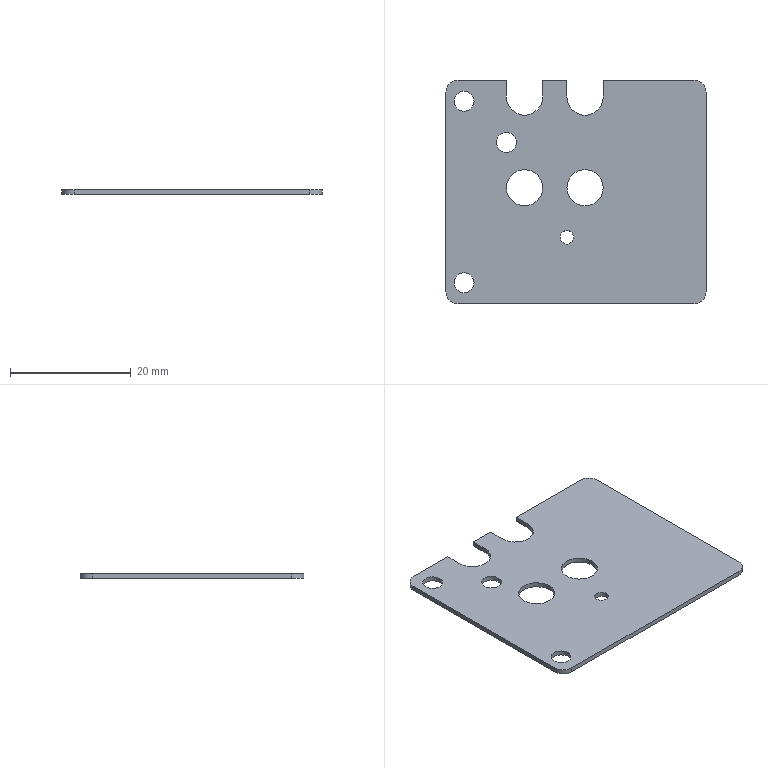Part | SolidWorks | features ICE 5, HoleWzd 2, Cut 1, Extrusion 1, Fillet 1, MirrorPattern 1, MoveFace 1 | 1 solid | 30 faces | box 43 x 37 x 0.8 mm | volume 1152 mm3 | cylinder 18 | plane 12 | commonest cylinder face diameters 3.3 x6 6 x6 4 x4 2.25 x2
STEP:
#1=CARTESIAN_POINT('',(-13.15,8.2,0.));
#2=VERTEX_POINT('',#1);
#3=CARTESIAN_POINT('',(-9.85,8.2,0.));
#4=VERTEX_POINT('',#3);
#5=CARTESIAN_POINT('',(-11.5,8.2,0.));
#6=DIRECTION('',(0.,0.,1.));
#7=DIRECTION('',(1.,0.,0.));
#8=AXIS2_PLACEMENT_3D('',#5,#6,#7);
#9=CIRCLE('',#8,1.65);
#10=EDGE_CURVE('',#2,#4,#9,.T.);
#11=ORIENTED_EDGE('',*,*,#10,.F.);
#12=CARTESIAN_POINT('',(-13.15,8.2,0.8));
#13=VERTEX_POINT('',#12);
#14=CARTESIAN_POINT('',(-13.15,8.2,-29.2));
#15=DIRECTION('',(0.,0.,1.));
#16=VECTOR('',#15,1000.);
#17=LINE('',#14,#16);
#18=EDGE_CURVE('',#2,#13,#17,.T.);
#19=ORIENTED_EDGE('',*,*,#18,.T.);
#20=CARTESIAN_POINT('',(-9.85,8.2,0.8));
#21=VERTEX_POINT('',#20);
#22=CARTESIAN_POINT('',(-11.5,8.2,0.8));
#23=DIRECTION('',(0.,0.,1.));
#24=DIRECTION('',(1.,0.,0.));
#25=AXIS2_PLACEMENT_3D('',#22,#23,#24);
#26=CIRCLE('',#25,1.65);
#27=EDGE_CURVE('',#13,#21,#26,.T.);
#28=ORIENTED_EDGE('',*,*,#27,.T.);
#29=CARTESIAN_POINT('',(-9.85,8.2,-29.2));
#30=DIRECTION('',(0.,0.,1.));
#31=VECTOR('',#30,1000.);
#32=LINE('',#29,#31);
#33=EDGE_CURVE('',#4,#21,#32,.T.);
#34=ORIENTED_EDGE('',*,*,#33,.F.);
#35=EDGE_LOOP('',(#11,#19,#28,#34));
#36=FACE_OUTER_BOUND('',#35,.T.);
#37=CARTESIAN_POINT('',(-11.5,8.2,-29.2));
#38=DIRECTION('',(0.,0.,1.));
#39=DIRECTION('',(1.,0.,0.));
#40=AXIS2_PLACEMENT_3D('',#37,#38,#39);
#41=CYLINDRICAL_SURFACE('',#40,1.65);
#42=ADVANCED_FACE('',(#36),#41,.F.);
#43=CARTESIAN_POINT('',(-20.15,15.,0.));
#44=VERTEX_POINT('',#43);
#45=CARTESIAN_POINT('',(-16.85,15.,0.));
#46=VERTEX_POINT('',#45);
#47=CARTESIAN_POINT('',(-18.5,15.,0.));
#48=DIRECTION('',(0.,0.,1.));
#49=DIRECTION('',(1.,0.,0.));
#50=AXIS2_PLACEMENT_3D('',#47,#48,#49);
#51=CIRCLE('',#50,1.65);
#52=EDGE_CURVE('',#44,#46,#51,.T.);
#53=ORIENTED_EDGE('',*,*,#52,.F.);
#54=CARTESIAN_POINT('',(-20.15,15.,0.8));
#55=VERTEX_POINT('',#54);
#56=CARTESIAN_POINT('',(-20.15,15.,0.8));
#57=DIRECTION('',(0.,0.,1.));
#58=VECTOR('',#57,1000.);
#59=LINE('',#56,#58);
#60=EDGE_CURVE('',#44,#55,#59,.T.);
#61=ORIENTED_EDGE('',*,*,#60,.T.);
#62=CARTESIAN_POINT('',(-16.85,15.,0.8));
#63=VERTEX_POINT('',#62);
#64=CARTESIAN_POINT('',(-18.5,15.,0.8));
#65=DIRECTION('',(0.,0.,1.));
#66=DIRECTION('',(1.,0.,0.));
#67=AXIS2_PLACEMENT_3D('',#64,#65,#66);
#68=CIRCLE('',#67,1.65);
#69=EDGE_CURVE('',#55,#63,#68,.T.);
#70=ORIENTED_EDGE('',*,*,#69,.T.);
#71=CARTESIAN_POINT('',(-16.85,15.,0.8));
#72=DIRECTION('',(0.,0.,1.));
#73=VECTOR('',#72,1000.);
#74=LINE('',#71,#73);
#75=EDGE_CURVE('',#46,#63,#74,.T.);
#76=ORIENTED_EDGE('',*,*,#75,.F.);
#77=EDGE_LOOP('',(#53,#61,#70,#76));
#78=FACE_OUTER_BOUND('',#77,.T.);
#79=CARTESIAN_POINT('',(-18.5,15.,0.8));
#80=DIRECTION('',(0.,0.,1.));
#81=DIRECTION('',(1.,0.,0.));
#82=AXIS2_PLACEMENT_3D('',#79,#80,#81);
#83=CYLINDRICAL_SURFACE('',#82,1.65);
#84=ADVANCED_FACE('',(#78),#83,.F.);
#85=CARTESIAN_POINT('',(-20.15,-15.,0.));
#86=VERTEX_POINT('',#85);
#87=CARTESIAN_POINT('',(-16.85,-15.,0.));
#88=VERTEX_POINT('',#87);
#89=CARTESIAN_POINT('',(-18.5,-15.,0.));
#90=DIRECTION('',(0.,0.,1.));
#91=DIRECTION('',(1.,0.,0.));
#92=AXIS2_PLACEMENT_3D('',#89,#90,#91);
#93=CIRCLE('',#92,1.65);
#94=EDGE_CURVE('',#86,#88,#93,.T.);
#95=ORIENTED_EDGE('',*,*,#94,.F.);
#96=CARTESIAN_POINT('',(-20.15,-15.,0.8));
#97=VERTEX_POINT('',#96);
#98=CARTESIAN_POINT('',(-20.15,-15.,0.8));
#99=DIRECTION('',(0.,0.,1.));
#100=VECTOR('',#99,1000.);
#101=LINE('',#98,#100);
#102=EDGE_CURVE('',#86,#97,#101,.T.);
#103=ORIENTED_EDGE('',*,*,#102,.T.);
#104=CARTESIAN_POINT('',(-16.85,-15.,0.8));
#105=VERTEX_POINT('',#104);
#106=CARTESIAN_POINT('',(-18.5,-15.,0.8));
#107=DIRECTION('',(0.,0.,1.));
#108=DIRECTION('',(1.,0.,0.));
#109=AXIS2_PLACEMENT_3D('',#106,#107,#108);
#110=CIRCLE('',#109,1.65);
#111=EDGE_CURVE('',#97,#105,#110,.T.);
#112=ORIENTED_EDGE('',*,*,#111,.T.);
#113=CARTESIAN_POINT('',(-16.85,-15.,0.8));
#114=DIRECTION('',(0.,0.,1.));
#115=VECTOR('',#114,1000.);
#116=LINE('',#113,#115);
#117=EDGE_CURVE('',#88,#105,#116,.T.);
#118=ORIENTED_EDGE('',*,*,#117,.F.);
#119=EDGE_LOOP('',(#95,#103,#112,#118));
#120=FACE_OUTER_BOUND('',#119,.T.);
#121=CARTESIAN_POINT('',(-18.5,-15.,0.8));
#122=DIRECTION('',(0.,0.,1.));
#123=DIRECTION('',(1.,0.,0.));
#124=AXIS2_PLACEMENT_3D('',#121,#122,#123);
#125=CYLINDRICAL_SURFACE('',#124,1.65);
#126=ADVANCED_FACE('',(#120),#125,.F.);
#127=CARTESIAN_POINT('',(-2.625,-7.5,0.));
#128=VERTEX_POINT('',#127);
#129=CARTESIAN_POINT('',(-0.375,-7.5,0.));
#130=VERTEX_POINT('',#129);
#131=CARTESIAN_POINT('',(-1.5,-7.5,0.));
#132=DIRECTION('',(0.,0.,1.));
#133=DIRECTION('',(1.,0.,0.));
#134=AXIS2_PLACEMENT_3D('',#131,#132,#133);
#135=CIRCLE('',#134,1.125);
#136=EDGE_CURVE('',#128,#130,#135,.T.);
#137=ORIENTED_EDGE('',*,*,#136,.F.);
#138=CARTESIAN_POINT('',(-2.625,-7.5,0.8));
#139=VERTEX_POINT('',#138);
#140=CARTESIAN_POINT('',(-2.625,-7.5,-1.2));
#141=DIRECTION('',(0.,0.,1.));
#142=VECTOR('',#141,1000.);
#143=LINE('',#140,#142);
#144=EDGE_CURVE('',#128,#139,#143,.T.);
#145=ORIENTED_EDGE('',*,*,#144,.T.);
#146=CARTESIAN_POINT('',(-0.375,-7.5,0.8));
#147=VERTEX_POINT('',#146);
#148=CARTESIAN_POINT('',(-1.5,-7.5,0.8));
#149=DIRECTION('',(0.,0.,1.));
#150=DIRECTION('',(1.,0.,0.));
#151=AXIS2_PLACEMENT_3D('',#148,#149,#150);
#152=CIRCLE('',#151,1.125);
#153=EDGE_CURVE('',#139,#147,#152,.T.);
#154=ORIENTED_EDGE('',*,*,#153,.T.);
#155=CARTESIAN_POINT('',(-0.375,-7.5,-1.2));
#156=DIRECTION('',(0.,0.,1.));
#157=VECTOR('',#156,1000.);
#158=LINE('',#155,#157);
#159=EDGE_CURVE('',#130,#147,#158,.T.);
#160=ORIENTED_EDGE('',*,*,#159,.F.);
#161=EDGE_LOOP('',(#137,#145,#154,#160));
#162=FACE_OUTER_BOUND('',#161,.T.);
#163=CARTESIAN_POINT('',(-1.5,-7.5,-1.2));
#164=DIRECTION('',(0.,0.,1.));
#165=DIRECTION('',(1.,0.,0.));
#166=AXIS2_PLACEMENT_3D('',#163,#164,#165);
#167=CYLINDRICAL_SURFACE('',#166,1.125);
#168=ADVANCED_FACE('',(#162),#167,.F.);
#169=CARTESIAN_POINT('',(-11.5,0.7,0.));
#170=VERTEX_POINT('',#169);
#171=CARTESIAN_POINT('',(-5.5,0.7,0.));
#172=VERTEX_POINT('',#171);
#173=CARTESIAN_POINT('',(-8.5,0.7,0.));
#174=DIRECTION('',(0.,0.,1.));
#175=DIRECTION('',(1.,0.,0.));
#176=AXIS2_PLACEMENT_3D('',#173,#174,#175);
#177=CIRCLE('',#176,3.);
#178=EDGE_CURVE('',#170,#172,#177,.T.);
#179=ORIENTED_EDGE('',*,*,#178,.F.);
#180=CARTESIAN_POINT('',(-11.5,0.7,0.8));
#181=VERTEX_POINT('',#180);
#182=CARTESIAN_POINT('',(-11.5,0.7,-1.2));
#183=DIRECTION('',(0.,0.,1.));
#184=VECTOR('',#183,1000.);
#185=LINE('',#182,#184);
#186=EDGE_CURVE('',#170,#181,#185,.T.);
#187=ORIENTED_EDGE('',*,*,#186,.T.);
#188=CARTESIAN_POINT('',(-5.5,0.7,0.8));
#189=VERTEX_POINT('',#188);
#190=CARTESIAN_POINT('',(-8.5,0.7,0.8));
#191=DIRECTION('',(0.,0.,1.));
#192=DIRECTION('',(1.,0.,0.));
#193=AXIS2_PLACEMENT_3D('',#190,#191,#192);
#194=CIRCLE('',#193,3.);
#195=EDGE_CURVE('',#181,#189,#194,.T.);
#196=ORIENTED_EDGE('',*,*,#195,.T.);
#197=CARTESIAN_POINT('',(-5.5,0.7,-1.2));
#198=DIRECTION('',(0.,0.,1.));
#199=VECTOR('',#198,1000.);
#200=LINE('',#197,#199);
#201=EDGE_CURVE('',#172,#189,#200,.T.);
#202=ORIENTED_EDGE('',*,*,#201,.F.);
#203=EDGE_LOOP('',(#179,#187,#196,#202));
#204=FACE_OUTER_BOUND('',#203,.T.);
#205=CARTESIAN_POINT('',(-8.5,0.7,-1.2));
#206=DIRECTION('',(0.,0.,1.));
#207=DIRECTION('',(1.,0.,0.));
#208=AXIS2_PLACEMENT_3D('',#205,#206,#207);
#209=CYLINDRICAL_SURFACE('',#208,3.);
#210=ADVANCED_FACE('',(#204),#209,.F.);
#211=CARTESIAN_POINT('',(-1.5,0.7,0.));
#212=VERTEX_POINT('',#211);
#213=CARTESIAN_POINT('',(4.5,0.7,0.));
#214=VERTEX_POINT('',#213);
#215=CARTESIAN_POINT('',(1.5,0.7,0.));
#216=DIRECTION('',(0.,0.,1.));
#217=DIRECTION('',(1.,0.,0.));
#218=AXIS2_PLACEMENT_3D('',#215,#216,#217);
#219=CIRCLE('',#218,3.);
#220=EDGE_CURVE('',#212,#214,#219,.T.);
#221=ORIENTED_EDGE('',*,*,#220,.F.);
#222=CARTESIAN_POINT('',(-1.5,0.7,0.8));
#223=VERTEX_POINT('',#222);
#224=CARTESIAN_POINT('',(-1.5,0.7,-1.2));
#225=DIRECTION('',(0.,0.,1.));
#226=VECTOR('',#225,1000.);
#227=LINE('',#224,#226);
#228=EDGE_CURVE('',#212,#223,#227,.T.);
#229=ORIENTED_EDGE('',*,*,#228,.T.);
#230=CARTESIAN_POINT('',(4.5,0.7,0.8));
#231=VERTEX_POINT('',#230);
#232=CARTESIAN_POINT('',(1.5,0.7,0.8));
#233=DIRECTION('',(0.,0.,1.));
#234=DIRECTION('',(1.,0.,0.));
#235=AXIS2_PLACEMENT_3D('',#232,#233,#234);
#236=CIRCLE('',#235,3.);
#237=EDGE_CURVE('',#223,#231,#236,.T.);
#238=ORIENTED_EDGE('',*,*,#237,.T.);
#239=CARTESIAN_POINT('',(4.5,0.7,-1.2));
#240=DIRECTION('',(0.,0.,1.));
#241=VECTOR('',#240,1000.);
#242=LINE('',#239,#241);
#243=EDGE_CURVE('',#214,#231,#242,.T.);
#244=ORIENTED_EDGE('',*,*,#243,.F.);
#245=EDGE_LOOP('',(#221,#229,#238,#244));
#246=FACE_OUTER_BOUND('',#245,.T.);
#247=CARTESIAN_POINT('',(1.5,0.7,-1.2));
#248=DIRECTION('',(0.,0.,1.));
#249=DIRECTION('',(1.,0.,0.));
#250=AXIS2_PLACEMENT_3D('',#247,#248,#249);
#251=CYLINDRICAL_SURFACE('',#250,3.);
#252=ADVANCED_FACE('',(#246),#251,.F.);
#253=CARTESIAN_POINT('',(-1.5,15.7,0.8));
#254=VERTEX_POINT('',#253);
#255=CARTESIAN_POINT('',(-1.5,15.7,0.));
#256=VERTEX_POINT('',#255);
#257=CARTESIAN_POINT('',(-1.5,15.7,-1.2));
#258=DIRECTION('',(0.,0.,-1.));
#259=VECTOR('',#258,1000.);
#260=LINE('',#257,#259);
#261=EDGE_CURVE('',#254,#256,#260,.T.);
#262=ORIENTED_EDGE('',*,*,#261,.F.);
#263=CARTESIAN_POINT('',(4.5,15.7,0.8));
#264=VERTEX_POINT('',#263);
#265=CARTESIAN_POINT('',(1.5,15.7,0.8));
#266=DIRECTION('',(0.,0.,1.));
#267=DIRECTION('',(1.,0.,0.));
#268=AXIS2_PLACEMENT_3D('',#265,#266,#267);
#269=CIRCLE('',#268,3.);
#270=EDGE_CURVE('',#254,#264,#269,.T.);
#271=ORIENTED_EDGE('',*,*,#270,.T.);
#272=CARTESIAN_POINT('',(4.5,15.7,0.));
#273=VERTEX_POINT('',#272);
#274=CARTESIAN_POINT('',(4.5,15.7,-1.2));
#275=DIRECTION('',(0.,0.,-1.));
#276=VECTOR('',#275,1000.);
#277=LINE('',#274,#276);
#278=EDGE_CURVE('',#264,#273,#277,.T.);
#279=ORIENTED_EDGE('',*,*,#278,.T.);
#280=CARTESIAN_POINT('',(1.5,15.7,0.));
#281=DIRECTION('',(0.,0.,1.));
#282=DIRECTION('',(1.,0.,0.));
#283=AXIS2_PLACEMENT_3D('',#280,#281,#282);
#284=CIRCLE('',#283,3.);
#285=EDGE_CURVE('',#256,#273,#284,.T.);
#286=ORIENTED_EDGE('',*,*,#285,.F.);
#287=EDGE_LOOP('',(#262,#271,#279,#286));
#288=FACE_OUTER_BOUND('',#287,.T.);
#289=CARTESIAN_POINT('',(1.5,15.7,-1.2));
#290=DIRECTION('',(0.,0.,1.));
#291=DIRECTION('',(1.,0.,0.));
#292=AXIS2_PLACEMENT_3D('',#289,#290,#291);
#293=CYLINDRICAL_SURFACE('',#292,3.);
#294=ADVANCED_FACE('',(#288),#293,.F.);
#295=CARTESIAN_POINT('',(-11.5,15.7,0.8));
#296=VERTEX_POINT('',#295);
#297=CARTESIAN_POINT('',(-11.5,15.7,0.));
#298=VERTEX_POINT('',#297);
#299=CARTESIAN_POINT('',(-11.5,15.7,-1.2));
#300=DIRECTION('',(0.,0.,-1.));
#301=VECTOR('',#300,1000.);
#302=LINE('',#299,#301);
#303=EDGE_CURVE('',#296,#298,#302,.T.);
#304=ORIENTED_EDGE('',*,*,#303,.F.);
#305=CARTESIAN_POINT('',(-5.5,15.7,0.8));
#306=VERTEX_POINT('',#305);
#307=CARTESIAN_POINT('',(-8.5,15.7,0.8));
#308=DIRECTION('',(0.,0.,1.));
#309=DIRECTION('',(1.,0.,0.));
#310=AXIS2_PLACEMENT_3D('',#307,#308,#309);
#311=CIRCLE('',#310,3.);
#312=EDGE_CURVE('',#296,#306,#311,.T.);
#313=ORIENTED_EDGE('',*,*,#312,.T.);
#314=CARTESIAN_POINT('',(-5.5,15.7,0.));
#315=VERTEX_POINT('',#314);
#316=CARTESIAN_POINT('',(-5.5,15.7,-1.2));
#317=DIRECTION('',(0.,0.,-1.));
#318=VECTOR('',#317,1000.);
#319=LINE('',#316,#318);
#320=EDGE_CURVE('',#306,#315,#319,.T.);
#321=ORIENTED_EDGE('',*,*,#320,.T.);
#322=CARTESIAN_POINT('',(-8.5,15.7,0.));
#323=DIRECTION('',(0.,0.,1.));
#324=DIRECTION('',(1.,0.,0.));
#325=AXIS2_PLACEMENT_3D('',#322,#323,#324);
#326=CIRCLE('',#325,3.);
#327=EDGE_CURVE('',#298,#315,#326,.T.);
#328=ORIENTED_EDGE('',*,*,#327,.F.);
#329=EDGE_LOOP('',(#304,#313,#321,#328));
#330=FACE_OUTER_BOUND('',#329,.T.);
#331=CARTESIAN_POINT('',(-8.5,15.7,-1.2));
#332=DIRECTION('',(0.,0.,1.));
#333=DIRECTION('',(1.,0.,0.));
#334=AXIS2_PLACEMENT_3D('',#331,#332,#333);
#335=CYLINDRICAL_SURFACE('',#334,3.);
#336=ADVANCED_FACE('',(#330),#335,.F.);
#337=CARTESIAN_POINT('',(19.5,18.5,0.8));
#338=VERTEX_POINT('',#337);
#339=CARTESIAN_POINT('',(4.5,18.5,0.8));
#340=VERTEX_POINT('',#339);
#341=CARTESIAN_POINT('',(-21.5,18.5,0.8));
#342=DIRECTION('',(-1.,0.,0.));
#343=VECTOR('',#342,1000.);
#344=LINE('',#341,#343);
#345=EDGE_CURVE('',#338,#340,#344,.T.);
#346=ORIENTED_EDGE('',*,*,#345,.F.);
#347=CARTESIAN_POINT('',(19.5,18.5,0.));
#348=VERTEX_POINT('',#347);
#349=CARTESIAN_POINT('',(19.5,18.5,0.8));
#350=DIRECTION('',(0.,0.,-1.));
#351=VECTOR('',#350,1000.);
#352=LINE('',#349,#351);
#353=EDGE_CURVE('',#338,#348,#352,.T.);
#354=ORIENTED_EDGE('',*,*,#353,.T.);
#355=CARTESIAN_POINT('',(4.5,18.5,0.));
#356=VERTEX_POINT('',#355);
#357=CARTESIAN_POINT('',(-21.5,18.5,0.));
#358=DIRECTION('',(-1.,0.,0.));
#359=VECTOR('',#358,1000.);
#360=LINE('',#357,#359);
#361=EDGE_CURVE('',#348,#356,#360,.T.);
#362=ORIENTED_EDGE('',*,*,#361,.T.);
#363=CARTESIAN_POINT('',(4.5,18.5,0.8));
#364=DIRECTION('',(0.,0.,1.));
#365=VECTOR('',#364,1000.);
#366=LINE('',#363,#365);
#367=EDGE_CURVE('',#356,#340,#366,.T.);
#368=ORIENTED_EDGE('',*,*,#367,.T.);
#369=EDGE_LOOP('',(#346,#354,#362,#368));
#370=FACE_OUTER_BOUND('',#369,.T.);
#371=CARTESIAN_POINT('',(-21.5,18.5,0.8));
#372=DIRECTION('',(0.,-1.,0.));
#373=DIRECTION('',(0.,0.,-1.));
#374=AXIS2_PLACEMENT_3D('',#371,#372,#373);
#375=PLANE('',#374);
#376=ADVANCED_FACE('',(#370),#375,.F.);
#377=CARTESIAN_POINT('',(-1.5,18.5,0.8));
#378=VERTEX_POINT('',#377);
#379=CARTESIAN_POINT('',(-5.5,18.5,0.8));
#380=VERTEX_POINT('',#379);
#381=CARTESIAN_POINT('',(-21.5,18.5,0.8));
#382=DIRECTION('',(-1.,0.,0.));
#383=VECTOR('',#382,1000.);
#384=LINE('',#381,#383);
#385=EDGE_CURVE('',#378,#380,#384,.T.);
#386=ORIENTED_EDGE('',*,*,#385,.F.);
#387=CARTESIAN_POINT('',(-1.5,18.5,0.));
#388=VERTEX_POINT('',#387);
#389=CARTESIAN_POINT('',(-1.5,18.5,0.8));
#390=DIRECTION('',(0.,0.,-1.));
#391=VECTOR('',#390,1000.);
#392=LINE('',#389,#391);
#393=EDGE_CURVE('',#378,#388,#392,.T.);
#394=ORIENTED_EDGE('',*,*,#393,.T.);
#395=CARTESIAN_POINT('',(-5.5,18.5,0.));
#396=VERTEX_POINT('',#395);
#397=CARTESIAN_POINT('',(-21.5,18.5,0.));
#398=DIRECTION('',(-1.,0.,0.));
#399=VECTOR('',#398,1000.);
#400=LINE('',#397,#399);
#401=EDGE_CURVE('',#388,#396,#400,.T.);
#402=ORIENTED_EDGE('',*,*,#401,.T.);
#403=CARTESIAN_POINT('',(-5.5,18.5,0.8));
#404=DIRECTION('',(0.,0.,1.));
#405=VECTOR('',#404,1000.);
#406=LINE('',#403,#405);
#407=EDGE_CURVE('',#396,#380,#406,.T.);
#408=ORIENTED_EDGE('',*,*,#407,.T.);
#409=EDGE_LOOP('',(#386,#394,#402,#408));
#410=FACE_OUTER_BOUND('',#409,.T.);
#411=CARTESIAN_POINT('',(-21.5,18.5,0.8));
#412=DIRECTION('',(0.,-1.,0.));
#413=DIRECTION('',(0.,0.,-1.));
#414=AXIS2_PLACEMENT_3D('',#411,#412,#413);
#415=PLANE('',#414);
#416=ADVANCED_FACE('',(#410),#415,.F.);
#417=CARTESIAN_POINT('',(21.5,-16.5,0.));
#418=VERTEX_POINT('',#417);
#419=CARTESIAN_POINT('',(21.5,16.5,0.));
#420=VERTEX_POINT('',#419);
#421=CARTESIAN_POINT('',(21.5,18.5,0.));
#422=DIRECTION('',(0.,1.,0.));
#423=VECTOR('',#422,1000.);
#424=LINE('',#421,#423);
#425=EDGE_CURVE('',#418,#420,#424,.T.);
#426=ORIENTED_EDGE('',*,*,#425,.T.);
#427=CARTESIAN_POINT('',(21.5,16.5,0.8));
#428=VERTEX_POINT('',#427);
#429=CARTESIAN_POINT('',(21.5,16.5,0.8));
#430=DIRECTION('',(0.,0.,1.));
#431=VECTOR('',#430,1000.);
#432=LINE('',#429,#431);
#433=EDGE_CURVE('',#420,#428,#432,.T.);
#434=ORIENTED_EDGE('',*,*,#433,.T.);
#435=CARTESIAN_POINT('',(21.5,-16.5,0.8));
#436=VERTEX_POINT('',#435);
#437=CARTESIAN_POINT('',(21.5,18.5,0.8));
#438=DIRECTION('',(0.,1.,0.));
#439=VECTOR('',#438,1000.);
#440=LINE('',#437,#439);
#441=EDGE_CURVE('',#436,#428,#440,.T.);
#442=ORIENTED_EDGE('',*,*,#441,.F.);
#443=CARTESIAN_POINT('',(21.5,-16.5,0.8));
#444=DIRECTION('',(0.,0.,-1.));
#445=VECTOR('',#444,1000.);
#446=LINE('',#443,#445);
#447=EDGE_CURVE('',#436,#418,#446,.T.);
#448=ORIENTED_EDGE('',*,*,#447,.T.);
#449=EDGE_LOOP('',(#426,#434,#442,#448));
#450=FACE_OUTER_BOUND('',#449,.T.);
#451=CARTESIAN_POINT('',(21.5,18.5,0.8));
#452=DIRECTION('',(-1.,0.,0.));
#453=DIRECTION('',(0.,-1.,0.));
#454=AXIS2_PLACEMENT_3D('',#451,#452,#453);
#455=PLANE('',#454);
#456=ADVANCED_FACE('',(#450),#455,.F.);
#457=CARTESIAN_POINT('',(-11.5,18.5,0.));
#458=VERTEX_POINT('',#457);
#459=CARTESIAN_POINT('',(-19.5,18.5,0.));
#460=VERTEX_POINT('',#459);
#461=CARTESIAN_POINT('',(-21.5,18.5,0.));
#462=DIRECTION('',(-1.,0.,0.));
#463=VECTOR('',#462,1000.);
#464=LINE('',#461,#463);
#465=EDGE_CURVE('',#458,#460,#464,.T.);
#466=ORIENTED_EDGE('',*,*,#465,.T.);
#467=CARTESIAN_POINT('',(-19.5,18.5,0.8));
#468=VERTEX_POINT('',#467);
#469=CARTESIAN_POINT('',(-19.5,18.5,0.8));
#470=DIRECTION('',(0.,0.,1.));
#471=VECTOR('',#470,1000.);
#472=LINE('',#469,#471);
#473=EDGE_CURVE('',#460,#468,#472,.T.);
#474=ORIENTED_EDGE('',*,*,#473,.T.);
#475=CARTESIAN_POINT('',(-11.5,18.5,0.8));
#476=VERTEX_POINT('',#475);
#477=CARTESIAN_POINT('',(-21.5,18.5,0.8));
#478=DIRECTION('',(-1.,0.,0.));
#479=VECTOR('',#478,1000.);
#480=LINE('',#477,#479);
#481=EDGE_CURVE('',#476,#468,#480,.T.);
#482=ORIENTED_EDGE('',*,*,#481,.F.);
#483=CARTESIAN_POINT('',(-11.5,18.5,0.8));
#484=DIRECTION('',(0.,0.,-1.));
#485=VECTOR('',#484,1000.);
#486=LINE('',#483,#485);
#487=EDGE_CURVE('',#476,#458,#486,.T.);
#488=ORIENTED_EDGE('',*,*,#487,.T.);
#489=EDGE_LOOP('',(#466,#474,#482,#488));
#490=FACE_OUTER_BOUND('',#489,.T.);
#491=CARTESIAN_POINT('',(-21.5,18.5,0.8));
#492=DIRECTION('',(0.,-1.,0.));
#493=DIRECTION('',(0.,0.,-1.));
#494=AXIS2_PLACEMENT_3D('',#491,#492,#493);
#495=PLANE('',#494);
#496=ADVANCED_FACE('',(#490),#495,.F.);
#497=CARTESIAN_POINT('',(-21.5,16.5,0.8));
#498=VERTEX_POINT('',#497);
#499=CARTESIAN_POINT('',(-21.5,-16.5,0.8));
#500=VERTEX_POINT('',#499);
#501=CARTESIAN_POINT('',(-21.5,18.5,0.8));
#502=DIRECTION('',(0.,-1.,0.));
#503=VECTOR('',#502,1000.);
#504=LINE('',#501,#503);
#505=EDGE_CURVE('',#498,#500,#504,.T.);
#506=ORIENTED_EDGE('',*,*,#505,.F.);
#507=CARTESIAN_POINT('',(-21.5,16.5,0.));
#508=VERTEX_POINT('',#507);
#509=CARTESIAN_POINT('',(-21.5,16.5,0.8));
#510=DIRECTION('',(0.,0.,-1.));
#511=VECTOR('',#510,1000.);
#512=LINE('',#509,#511);
#513=EDGE_CURVE('',#498,#508,#512,.T.);
#514=ORIENTED_EDGE('',*,*,#513,.T.);
#515=CARTESIAN_POINT('',(-21.5,-16.5,0.));
#516=VERTEX_POINT('',#515);
#517=CARTESIAN_POINT('',(-21.5,18.5,0.));
#518=DIRECTION('',(0.,-1.,0.));
#519=VECTOR('',#518,1000.);
#520=LINE('',#517,#519);
#521=EDGE_CURVE('',#508,#516,#520,.T.);
#522=ORIENTED_EDGE('',*,*,#521,.T.);
#523=CARTESIAN_POINT('',(-21.5,-16.5,0.8));
#524=DIRECTION('',(0.,0.,1.));
#525=VECTOR('',#524,1000.);
#526=LINE('',#523,#525);
#527=EDGE_CURVE('',#516,#500,#526,.T.);
#528=ORIENTED_EDGE('',*,*,#527,.T.);
#529=EDGE_LOOP('',(#506,#514,#522,#528));
#530=FACE_OUTER_BOUND('',#529,.T.);
#531=CARTESIAN_POINT('',(-21.5,18.5,0.8));
#532=DIRECTION('',(1.,0.,0.));
#533=DIRECTION('',(0.,1.,0.));
#534=AXIS2_PLACEMENT_3D('',#531,#532,#533);
#535=PLANE('',#534);
#536=ADVANCED_FACE('',(#530),#535,.F.);
#537=CARTESIAN_POINT('',(-19.5,-18.5,0.8));
#538=VERTEX_POINT('',#537);
#539=CARTESIAN_POINT('',(19.5,-18.5,0.8));
#540=VERTEX_POINT('',#539);
#541=CARTESIAN_POINT('',(-21.5,-18.5,0.8));
#542=DIRECTION('',(1.,0.,0.));
#543=VECTOR('',#542,1000.);
#544=LINE('',#541,#543);
#545=EDGE_CURVE('',#538,#540,#544,.T.);
#546=ORIENTED_EDGE('',*,*,#545,.F.);
#547=CARTESIAN_POINT('',(-19.5,-18.5,0.));
#548=VERTEX_POINT('',#547);
#549=CARTESIAN_POINT('',(-19.5,-18.5,0.8));
#550=DIRECTION('',(0.,0.,-1.));
#551=VECTOR('',#550,1000.);
#552=LINE('',#549,#551);
#553=EDGE_CURVE('',#538,#548,#552,.T.);
#554=ORIENTED_EDGE('',*,*,#553,.T.);
#555=CARTESIAN_POINT('',(19.5,-18.5,0.));
#556=VERTEX_POINT('',#555);
#557=CARTESIAN_POINT('',(-21.5,-18.5,0.));
#558=DIRECTION('',(1.,0.,0.));
#559=VECTOR('',#558,1000.);
#560=LINE('',#557,#559);
#561=EDGE_CURVE('',#548,#556,#560,.T.);
#562=ORIENTED_EDGE('',*,*,#561,.T.);
#563=CARTESIAN_POINT('',(19.5,-18.5,0.8));
#564=DIRECTION('',(0.,0.,1.));
#565=VECTOR('',#564,1000.);
#566=LINE('',#563,#565);
#567=EDGE_CURVE('',#556,#540,#566,.T.);
#568=ORIENTED_EDGE('',*,*,#567,.T.);
#569=EDGE_LOOP('',(#546,#554,#562,#568));
#570=FACE_OUTER_BOUND('',#569,.T.);
#571=CARTESIAN_POINT('',(-21.5,-18.5,0.8));
#572=DIRECTION('',(0.,1.,0.));
#573=DIRECTION('',(0.,0.,1.));
#574=AXIS2_PLACEMENT_3D('',#571,#572,#573);
#575=PLANE('',#574);
#576=ADVANCED_FACE('',(#570),#575,.F.);
#577=CARTESIAN_POINT('',(-11.5,8.2,0.8));
#578=DIRECTION('',(0.,0.,1.));
#579=DIRECTION('',(1.,0.,0.));
#580=AXIS2_PLACEMENT_3D('',#577,#578,#579);
#581=CIRCLE('',#580,1.65);
#582=EDGE_CURVE('',#21,#13,#581,.T.);
#583=ORIENTED_EDGE('',*,*,#582,.F.);
#584=ORIENTED_EDGE('',*,*,#27,.F.);
#585=EDGE_LOOP('',(#583,#584));
#586=FACE_BOUND('',#585,.T.);
#587=CARTESIAN_POINT('',(-18.5,15.,0.8));
#588=DIRECTION('',(0.,0.,1.));
#589=DIRECTION('',(1.,0.,0.));
#590=AXIS2_PLACEMENT_3D('',#587,#588,#589);
#591=CIRCLE('',#590,1.65);
#592=EDGE_CURVE('',#63,#55,#591,.T.);
#593=ORIENTED_EDGE('',*,*,#592,.F.);
#594=ORIENTED_EDGE('',*,*,#69,.F.);
#595=EDGE_LOOP('',(#593,#594));
#596=FACE_BOUND('',#595,.T.);
#597=CARTESIAN_POINT('',(-18.5,-15.,0.8));
#598=DIRECTION('',(0.,0.,1.));
#599=DIRECTION('',(1.,0.,0.));
#600=AXIS2_PLACEMENT_3D('',#597,#598,#599);
#601=CIRCLE('',#600,1.65);
#602=EDGE_CURVE('',#105,#97,#601,.T.);
#603=ORIENTED_EDGE('',*,*,#602,.F.);
#604=ORIENTED_EDGE('',*,*,#111,.F.);
#605=EDGE_LOOP('',(#603,#604));
#606=FACE_BOUND('',#605,.T.);
#607=ORIENTED_EDGE('',*,*,#441,.T.);
#608=CARTESIAN_POINT('',(19.5,16.5,0.8));
#609=DIRECTION('',(0.,0.,1.));
#610=DIRECTION('',(1.,0.,0.));
#611=AXIS2_PLACEMENT_3D('',#608,#609,#610);
#612=CIRCLE('',#611,2.);
#613=EDGE_CURVE('',#428,#338,#612,.T.);
#614=ORIENTED_EDGE('',*,*,#613,.T.);
#615=ORIENTED_EDGE('',*,*,#345,.T.);
#616=CARTESIAN_POINT('',(4.5,15.7,0.8));
#617=DIRECTION('',(0.,1.,0.));
#618=VECTOR('',#617,1000.);
#619=LINE('',#616,#618);
#620=EDGE_CURVE('',#264,#340,#619,.T.);
#621=ORIENTED_EDGE('',*,*,#620,.F.);
#622=ORIENTED_EDGE('',*,*,#270,.F.);
#623=CARTESIAN_POINT('',(-1.5,15.7,0.8));
#624=DIRECTION('',(0.,-1.,0.));
#625=VECTOR('',#624,1000.);
#626=LINE('',#623,#625);
#627=EDGE_CURVE('',#378,#254,#626,.T.);
#628=ORIENTED_EDGE('',*,*,#627,.F.);
#629=ORIENTED_EDGE('',*,*,#385,.T.);
#630=CARTESIAN_POINT('',(-5.5,15.7,0.8));
#631=DIRECTION('',(0.,1.,0.));
#632=VECTOR('',#631,1000.);
#633=LINE('',#630,#632);
#634=EDGE_CURVE('',#306,#380,#633,.T.);
#635=ORIENTED_EDGE('',*,*,#634,.F.);
#636=ORIENTED_EDGE('',*,*,#312,.F.);
#637=CARTESIAN_POINT('',(-11.5,15.7,0.8));
#638=DIRECTION('',(0.,-1.,0.));
#639=VECTOR('',#638,1000.);
#640=LINE('',#637,#639);
#641=EDGE_CURVE('',#476,#296,#640,.T.);
#642=ORIENTED_EDGE('',*,*,#641,.F.);
#643=ORIENTED_EDGE('',*,*,#481,.T.);
#644=CARTESIAN_POINT('',(-19.5,16.5,0.8));
#645=DIRECTION('',(0.,0.,1.));
#646=DIRECTION('',(1.,0.,0.));
#647=AXIS2_PLACEMENT_3D('',#644,#645,#646);
#648=CIRCLE('',#647,2.);
#649=EDGE_CURVE('',#468,#498,#648,.T.);
#650=ORIENTED_EDGE('',*,*,#649,.T.);
#651=ORIENTED_EDGE('',*,*,#505,.T.);
#652=CARTESIAN_POINT('',(-19.5,-16.5,0.8));
#653=DIRECTION('',(0.,0.,1.));
#654=DIRECTION('',(1.,0.,0.));
#655=AXIS2_PLACEMENT_3D('',#652,#653,#654);
#656=CIRCLE('',#655,2.);
#657=EDGE_CURVE('',#500,#538,#656,.T.);
#658=ORIENTED_EDGE('',*,*,#657,.T.);
#659=ORIENTED_EDGE('',*,*,#545,.T.);
#660=CARTESIAN_POINT('',(19.5,-16.5,0.8));
#661=DIRECTION('',(0.,0.,1.));
#662=DIRECTION('',(1.,0.,0.));
#663=AXIS2_PLACEMENT_3D('',#660,#661,#662);
#664=CIRCLE('',#663,2.);
#665=EDGE_CURVE('',#540,#436,#664,.T.);
#666=ORIENTED_EDGE('',*,*,#665,.T.);
#667=EDGE_LOOP('',(#607,#614,#615,#621,#622,#628,#629,#635,#636,#642,#643,#650,#651,#658,#659,#666));
#668=FACE_OUTER_BOUND('',#667,.T.);
#669=CARTESIAN_POINT('',(-1.5,-7.5,0.8));
#670=DIRECTION('',(0.,0.,1.));
#671=DIRECTION('',(1.,0.,0.));
#672=AXIS2_PLACEMENT_3D('',#669,#670,#671);
#673=CIRCLE('',#672,1.125);
#674=EDGE_CURVE('',#147,#139,#673,.T.);
#675=ORIENTED_EDGE('',*,*,#674,.F.);
#676=ORIENTED_EDGE('',*,*,#153,.F.);
#677=EDGE_LOOP('',(#675,#676));
#678=FACE_BOUND('',#677,.T.);
#679=CARTESIAN_POINT('',(-8.5,0.7,0.8));
#680=DIRECTION('',(0.,0.,1.));
#681=DIRECTION('',(1.,0.,0.));
#682=AXIS2_PLACEMENT_3D('',#679,#680,#681);
#683=CIRCLE('',#682,3.);
#684=EDGE_CURVE('',#189,#181,#683,.T.);
#685=ORIENTED_EDGE('',*,*,#684,.F.);
#686=ORIENTED_EDGE('',*,*,#195,.F.);
#687=EDGE_LOOP('',(#685,#686));
#688=FACE_BOUND('',#687,.T.);
#689=CARTESIAN_POINT('',(1.5,0.7,0.8));
#690=DIRECTION('',(0.,0.,1.));
#691=DIRECTION('',(1.,0.,0.));
#692=AXIS2_PLACEMENT_3D('',#689,#690,#691);
#693=CIRCLE('',#692,3.);
#694=EDGE_CURVE('',#231,#223,#693,.T.);
#695=ORIENTED_EDGE('',*,*,#694,.F.);
#696=ORIENTED_EDGE('',*,*,#237,.F.);
#697=EDGE_LOOP('',(#695,#696));
#698=FACE_BOUND('',#697,.T.);
#699=CARTESIAN_POINT('',(0.,0.,0.8));
#700=DIRECTION('',(0.,0.,1.));
#701=DIRECTION('',(1.,0.,0.));
#702=AXIS2_PLACEMENT_3D('',#699,#700,#701);
#703=PLANE('',#702);
#704=ADVANCED_FACE('',(#586,#596,#606,#668,#678,#688,#698),#703,.T.);
#705=CARTESIAN_POINT('',(-11.5,8.2,0.));
#706=DIRECTION('',(0.,0.,1.));
#707=DIRECTION('',(1.,0.,0.));
#708=AXIS2_PLACEMENT_3D('',#705,#706,#707);
#709=CIRCLE('',#708,1.65);
#710=EDGE_CURVE('',#4,#2,#709,.T.);
#711=ORIENTED_EDGE('',*,*,#710,.T.);
#712=ORIENTED_EDGE('',*,*,#10,.T.);
#713=EDGE_LOOP('',(#711,#712));
#714=FACE_BOUND('',#713,.T.);
#715=CARTESIAN_POINT('',(-18.5,15.,0.));
#716=DIRECTION('',(0.,0.,1.));
#717=DIRECTION('',(1.,0.,0.));
#718=AXIS2_PLACEMENT_3D('',#715,#716,#717);
#719=CIRCLE('',#718,1.65);
#720=EDGE_CURVE('',#46,#44,#719,.T.);
#721=ORIENTED_EDGE('',*,*,#720,.T.);
#722=ORIENTED_EDGE('',*,*,#52,.T.);
#723=EDGE_LOOP('',(#721,#722));
#724=FACE_BOUND('',#723,.T.);
#725=CARTESIAN_POINT('',(-18.5,-15.,0.));
#726=DIRECTION('',(0.,0.,1.));
#727=DIRECTION('',(1.,0.,0.));
#728=AXIS2_PLACEMENT_3D('',#725,#726,#727);
#729=CIRCLE('',#728,1.65);
#730=EDGE_CURVE('',#88,#86,#729,.T.);
#731=ORIENTED_EDGE('',*,*,#730,.T.);
#732=ORIENTED_EDGE('',*,*,#94,.T.);
#733=EDGE_LOOP('',(#731,#732));
#734=FACE_BOUND('',#733,.T.);
#735=CARTESIAN_POINT('',(-1.5,-7.5,0.));
#736=DIRECTION('',(0.,0.,1.));
#737=DIRECTION('',(1.,0.,0.));
#738=AXIS2_PLACEMENT_3D('',#735,#736,#737);
#739=CIRCLE('',#738,1.125);
#740=EDGE_CURVE('',#130,#128,#739,.T.);
#741=ORIENTED_EDGE('',*,*,#740,.T.);
#742=ORIENTED_EDGE('',*,*,#136,.T.);
#743=EDGE_LOOP('',(#741,#742));
#744=FACE_BOUND('',#743,.T.);
#745=CARTESIAN_POINT('',(-8.5,0.7,0.));
#746=DIRECTION('',(0.,0.,1.));
#747=DIRECTION('',(1.,0.,0.));
#748=AXIS2_PLACEMENT_3D('',#745,#746,#747);
#749=CIRCLE('',#748,3.);
#750=EDGE_CURVE('',#172,#170,#749,.T.);
#751=ORIENTED_EDGE('',*,*,#750,.T.);
#752=ORIENTED_EDGE('',*,*,#178,.T.);
#753=EDGE_LOOP('',(#751,#752));
#754=FACE_BOUND('',#753,.T.);
#755=CARTESIAN_POINT('',(1.5,0.7,0.));
#756=DIRECTION('',(0.,0.,1.));
#757=DIRECTION('',(1.,0.,0.));
#758=AXIS2_PLACEMENT_3D('',#755,#756,#757);
#759=CIRCLE('',#758,3.);
#760=EDGE_CURVE('',#214,#212,#759,.T.);
#761=ORIENTED_EDGE('',*,*,#760,.T.);
#762=ORIENTED_EDGE('',*,*,#220,.T.);
#763=EDGE_LOOP('',(#761,#762));
#764=FACE_BOUND('',#763,.T.);
#765=ORIENTED_EDGE('',*,*,#361,.F.);
#766=CARTESIAN_POINT('',(19.5,16.5,0.));
#767=DIRECTION('',(0.,0.,-1.));
#768=DIRECTION('',(1.,0.,0.));
#769=AXIS2_PLACEMENT_3D('',#766,#767,#768);
#770=CIRCLE('',#769,2.);
#771=EDGE_CURVE('',#348,#420,#770,.T.);
#772=ORIENTED_EDGE('',*,*,#771,.T.);
#773=ORIENTED_EDGE('',*,*,#425,.F.);
#774=CARTESIAN_POINT('',(19.5,-16.5,0.));
#775=DIRECTION('',(0.,0.,-1.));
#776=DIRECTION('',(1.,0.,0.));
#777=AXIS2_PLACEMENT_3D('',#774,#775,#776);
#778=CIRCLE('',#777,2.);
#779=EDGE_CURVE('',#418,#556,#778,.T.);
#780=ORIENTED_EDGE('',*,*,#779,.T.);
#781=ORIENTED_EDGE('',*,*,#561,.F.);
#782=CARTESIAN_POINT('',(-19.5,-16.5,0.));
#783=DIRECTION('',(0.,0.,-1.));
#784=DIRECTION('',(1.,0.,0.));
#785=AXIS2_PLACEMENT_3D('',#782,#783,#784);
#786=CIRCLE('',#785,2.);
#787=EDGE_CURVE('',#548,#516,#786,.T.);
#788=ORIENTED_EDGE('',*,*,#787,.T.);
#789=ORIENTED_EDGE('',*,*,#521,.F.);
#790=CARTESIAN_POINT('',(-19.5,16.5,0.));
#791=DIRECTION('',(0.,0.,-1.));
#792=DIRECTION('',(1.,0.,0.));
#793=AXIS2_PLACEMENT_3D('',#790,#791,#792);
#794=CIRCLE('',#793,2.);
#795=EDGE_CURVE('',#508,#460,#794,.T.);
#796=ORIENTED_EDGE('',*,*,#795,.T.);
#797=ORIENTED_EDGE('',*,*,#465,.F.);
#798=CARTESIAN_POINT('',(-11.5,0.,0.));
#799=DIRECTION('',(0.,-1.,0.));
#800=VECTOR('',#799,1000.);
#801=LINE('',#798,#800);
#802=EDGE_CURVE('',#458,#298,#801,.T.);
#803=ORIENTED_EDGE('',*,*,#802,.T.);
#804=ORIENTED_EDGE('',*,*,#327,.T.);
#805=CARTESIAN_POINT('',(-5.5,0.,0.));
#806=DIRECTION('',(0.,1.,0.));
#807=VECTOR('',#806,1000.);
#808=LINE('',#805,#807);
#809=EDGE_CURVE('',#315,#396,#808,.T.);
#810=ORIENTED_EDGE('',*,*,#809,.T.);
#811=ORIENTED_EDGE('',*,*,#401,.F.);
#812=CARTESIAN_POINT('',(-1.5,0.,0.));
#813=DIRECTION('',(0.,-1.,0.));
#814=VECTOR('',#813,1000.);
#815=LINE('',#812,#814);
#816=EDGE_CURVE('',#388,#256,#815,.T.);
#817=ORIENTED_EDGE('',*,*,#816,.T.);
#818=ORIENTED_EDGE('',*,*,#285,.T.);
#819=CARTESIAN_POINT('',(4.5,0.,0.));
#820=DIRECTION('',(0.,1.,0.));
#821=VECTOR('',#820,1000.);
#822=LINE('',#819,#821);
#823=EDGE_CURVE('',#273,#356,#822,.T.);
#824=ORIENTED_EDGE('',*,*,#823,.T.);
#825=EDGE_LOOP('',(#765,#772,#773,#780,#781,#788,#789,#796,#797,#803,#804,#810,#811,#817,#818,#824));
#826=FACE_OUTER_BOUND('',#825,.T.);
#827=CARTESIAN_POINT('',(0.,0.,0.));
#828=DIRECTION('',(0.,0.,1.));
#829=DIRECTION('',(1.,0.,0.));
#830=AXIS2_PLACEMENT_3D('',#827,#828,#829);
#831=PLANE('',#830);
#832=ADVANCED_FACE('',(#714,#724,#734,#744,#754,#764,#826),#831,.F.);
#833=ORIENTED_EDGE('',*,*,#228,.F.);
#834=ORIENTED_EDGE('',*,*,#760,.F.);
#835=ORIENTED_EDGE('',*,*,#243,.T.);
#836=ORIENTED_EDGE('',*,*,#694,.T.);
#837=EDGE_LOOP('',(#833,#834,#835,#836));
#838=FACE_OUTER_BOUND('',#837,.T.);
#839=CARTESIAN_POINT('',(1.5,0.7,-1.2));
#840=DIRECTION('',(0.,0.,1.));
#841=DIRECTION('',(1.,0.,0.));
#842=AXIS2_PLACEMENT_3D('',#839,#840,#841);
#843=CYLINDRICAL_SURFACE('',#842,3.);
#844=ADVANCED_FACE('',(#838),#843,.F.);
#845=ORIENTED_EDGE('',*,*,#186,.F.);
#846=ORIENTED_EDGE('',*,*,#750,.F.);
#847=ORIENTED_EDGE('',*,*,#201,.T.);
#848=ORIENTED_EDGE('',*,*,#684,.T.);
#849=EDGE_LOOP('',(#845,#846,#847,#848));
#850=FACE_OUTER_BOUND('',#849,.T.);
#851=CARTESIAN_POINT('',(-8.5,0.7,-1.2));
#852=DIRECTION('',(0.,0.,1.));
#853=DIRECTION('',(1.,0.,0.));
#854=AXIS2_PLACEMENT_3D('',#851,#852,#853);
#855=CYLINDRICAL_SURFACE('',#854,3.);
#856=ADVANCED_FACE('',(#850),#855,.F.);
#857=ORIENTED_EDGE('',*,*,#144,.F.);
#858=ORIENTED_EDGE('',*,*,#740,.F.);
#859=ORIENTED_EDGE('',*,*,#159,.T.);
#860=ORIENTED_EDGE('',*,*,#674,.T.);
#861=EDGE_LOOP('',(#857,#858,#859,#860));
#862=FACE_OUTER_BOUND('',#861,.T.);
#863=CARTESIAN_POINT('',(-1.5,-7.5,-1.2));
#864=DIRECTION('',(0.,0.,1.));
#865=DIRECTION('',(1.,0.,0.));
#866=AXIS2_PLACEMENT_3D('',#863,#864,#865);
#867=CYLINDRICAL_SURFACE('',#866,1.125);
#868=ADVANCED_FACE('',(#862),#867,.F.);
#869=ORIENTED_EDGE('',*,*,#809,.F.);
#870=ORIENTED_EDGE('',*,*,#320,.F.);
#871=ORIENTED_EDGE('',*,*,#634,.T.);
#872=ORIENTED_EDGE('',*,*,#407,.F.);
#873=EDGE_LOOP('',(#869,#870,#871,#872));
#874=FACE_OUTER_BOUND('',#873,.T.);
#875=CARTESIAN_POINT('',(-5.5,15.7,-8.2));
#876=DIRECTION('',(1.,0.,0.));
#877=DIRECTION('',(0.,0.,-1.));
#878=AXIS2_PLACEMENT_3D('',#875,#876,#877);
#879=PLANE('',#878);
#880=ADVANCED_FACE('',(#874),#879,.F.);
#881=ORIENTED_EDGE('',*,*,#641,.T.);
#882=ORIENTED_EDGE('',*,*,#303,.T.);
#883=ORIENTED_EDGE('',*,*,#802,.F.);
#884=ORIENTED_EDGE('',*,*,#487,.F.);
#885=EDGE_LOOP('',(#881,#882,#883,#884));
#886=FACE_OUTER_BOUND('',#885,.T.);
#887=CARTESIAN_POINT('',(-11.5,15.7,-8.2));
#888=DIRECTION('',(-1.,0.,0.));
#889=DIRECTION('',(0.,0.,1.));
#890=AXIS2_PLACEMENT_3D('',#887,#888,#889);
#891=PLANE('',#890);
#892=ADVANCED_FACE('',(#886),#891,.F.);
#893=ORIENTED_EDGE('',*,*,#823,.F.);
#894=ORIENTED_EDGE('',*,*,#278,.F.);
#895=ORIENTED_EDGE('',*,*,#620,.T.);
#896=ORIENTED_EDGE('',*,*,#367,.F.);
#897=EDGE_LOOP('',(#893,#894,#895,#896));
#898=FACE_OUTER_BOUND('',#897,.T.);
#899=CARTESIAN_POINT('',(4.5,15.7,-8.2));
#900=DIRECTION('',(1.,0.,0.));
#901=DIRECTION('',(0.,0.,-1.));
#902=AXIS2_PLACEMENT_3D('',#899,#900,#901);
#903=PLANE('',#902);
#904=ADVANCED_FACE('',(#898),#903,.F.);
#905=ORIENTED_EDGE('',*,*,#627,.T.);
#906=ORIENTED_EDGE('',*,*,#261,.T.);
#907=ORIENTED_EDGE('',*,*,#816,.F.);
#908=ORIENTED_EDGE('',*,*,#393,.F.);
#909=EDGE_LOOP('',(#905,#906,#907,#908));
#910=FACE_OUTER_BOUND('',#909,.T.);
#911=CARTESIAN_POINT('',(-1.5,15.7,-8.2));
#912=DIRECTION('',(-1.,0.,0.));
#913=DIRECTION('',(0.,0.,1.));
#914=AXIS2_PLACEMENT_3D('',#911,#912,#913);
#915=PLANE('',#914);
#916=ADVANCED_FACE('',(#910),#915,.F.);
#917=ORIENTED_EDGE('',*,*,#102,.F.);
#918=ORIENTED_EDGE('',*,*,#730,.F.);
#919=ORIENTED_EDGE('',*,*,#117,.T.);
#920=ORIENTED_EDGE('',*,*,#602,.T.);
#921=EDGE_LOOP('',(#917,#918,#919,#920));
#922=FACE_OUTER_BOUND('',#921,.T.);
#923=CARTESIAN_POINT('',(-18.5,-15.,0.8));
#924=DIRECTION('',(0.,0.,1.));
#925=DIRECTION('',(1.,0.,0.));
#926=AXIS2_PLACEMENT_3D('',#923,#924,#925);
#927=CYLINDRICAL_SURFACE('',#926,1.65);
#928=ADVANCED_FACE('',(#922),#927,.F.);
#929=ORIENTED_EDGE('',*,*,#60,.F.);
#930=ORIENTED_EDGE('',*,*,#720,.F.);
#931=ORIENTED_EDGE('',*,*,#75,.T.);
#932=ORIENTED_EDGE('',*,*,#592,.T.);
#933=EDGE_LOOP('',(#929,#930,#931,#932));
#934=FACE_OUTER_BOUND('',#933,.T.);
#935=CARTESIAN_POINT('',(-18.5,15.,0.8));
#936=DIRECTION('',(0.,0.,1.));
#937=DIRECTION('',(1.,0.,0.));
#938=AXIS2_PLACEMENT_3D('',#935,#936,#937);
#939=CYLINDRICAL_SURFACE('',#938,1.65);
#940=ADVANCED_FACE('',(#934),#939,.F.);
#941=ORIENTED_EDGE('',*,*,#613,.F.);
#942=ORIENTED_EDGE('',*,*,#433,.F.);
#943=ORIENTED_EDGE('',*,*,#771,.F.);
#944=ORIENTED_EDGE('',*,*,#353,.F.);
#945=EDGE_LOOP('',(#941,#942,#943,#944));
#946=FACE_OUTER_BOUND('',#945,.T.);
#947=CARTESIAN_POINT('',(19.5,16.5,0.8));
#948=DIRECTION('',(0.,0.,-1.));
#949=DIRECTION('',(-1.,0.,0.));
#950=AXIS2_PLACEMENT_3D('',#947,#948,#949);
#951=CYLINDRICAL_SURFACE('',#950,2.);
#952=ADVANCED_FACE('',(#946),#951,.T.);
#953=ORIENTED_EDGE('',*,*,#649,.F.);
#954=ORIENTED_EDGE('',*,*,#473,.F.);
#955=ORIENTED_EDGE('',*,*,#795,.F.);
#956=ORIENTED_EDGE('',*,*,#513,.F.);
#957=EDGE_LOOP('',(#953,#954,#955,#956));
#958=FACE_OUTER_BOUND('',#957,.T.);
#959=CARTESIAN_POINT('',(-19.5,16.5,0.8));
#960=DIRECTION('',(0.,0.,-1.));
#961=DIRECTION('',(-1.,0.,0.));
#962=AXIS2_PLACEMENT_3D('',#959,#960,#961);
#963=CYLINDRICAL_SURFACE('',#962,2.);
#964=ADVANCED_FACE('',(#958),#963,.T.);
#965=ORIENTED_EDGE('',*,*,#657,.F.);
#966=ORIENTED_EDGE('',*,*,#527,.F.);
#967=ORIENTED_EDGE('',*,*,#787,.F.);
#968=ORIENTED_EDGE('',*,*,#553,.F.);
#969=EDGE_LOOP('',(#965,#966,#967,#968));
#970=FACE_OUTER_BOUND('',#969,.T.);
#971=CARTESIAN_POINT('',(-19.5,-16.5,0.8));
#972=DIRECTION('',(0.,0.,-1.));
#973=DIRECTION('',(-1.,0.,0.));
#974=AXIS2_PLACEMENT_3D('',#971,#972,#973);
#975=CYLINDRICAL_SURFACE('',#974,2.);
#976=ADVANCED_FACE('',(#970),#975,.T.);
#977=ORIENTED_EDGE('',*,*,#665,.F.);
#978=ORIENTED_EDGE('',*,*,#567,.F.);
#979=ORIENTED_EDGE('',*,*,#779,.F.);
#980=ORIENTED_EDGE('',*,*,#447,.F.);
#981=EDGE_LOOP('',(#977,#978,#979,#980));
#982=FACE_OUTER_BOUND('',#981,.T.);
#983=CARTESIAN_POINT('',(19.5,-16.5,0.8));
#984=DIRECTION('',(0.,0.,-1.));
#985=DIRECTION('',(-1.,0.,0.));
#986=AXIS2_PLACEMENT_3D('',#983,#984,#985);
#987=CYLINDRICAL_SURFACE('',#986,2.);
#988=ADVANCED_FACE('',(#982),#987,.T.);
#989=ORIENTED_EDGE('',*,*,#18,.F.);
#990=ORIENTED_EDGE('',*,*,#710,.F.);
#991=ORIENTED_EDGE('',*,*,#33,.T.);
#992=ORIENTED_EDGE('',*,*,#582,.T.);
#993=EDGE_LOOP('',(#989,#990,#991,#992));
#994=FACE_OUTER_BOUND('',#993,.T.);
#995=CARTESIAN_POINT('',(-11.5,8.2,-29.2));
#996=DIRECTION('',(0.,0.,1.));
#997=DIRECTION('',(1.,0.,0.));
#998=AXIS2_PLACEMENT_3D('',#995,#996,#997);
#999=CYLINDRICAL_SURFACE('',#998,1.65);
#1000=ADVANCED_FACE('',(#994),#999,.F.);
#1001=CLOSED_SHELL('',(#42,#84,#126,#168,#210,#252,#294,#336,#376,#416,#456,#496,#536,#576,#704,#832,#844,#856,#868,#880,#892,#904,#916,#928,#940,#952,#964,#976,#988,#1000));
#1002=MANIFOLD_SOLID_BREP('',#1001);
#1003=CARTESIAN_POINT('',(0.,0.,0.));
#1004=DIRECTION('',(0.,0.,1.));
#1005=DIRECTION('',(1.,0.,0.));
#1006=AXIS2_PLACEMENT_3D('',#1003,#1004,#1005);
#1007=(LENGTH_UNIT()NAMED_UNIT(*)SI_UNIT(.MILLI.,.METRE.));
#1008=UNCERTAINTY_MEASURE_WITH_UNIT(LENGTH_MEASURE(0.00001),#1007,'','');
#1009=(NAMED_UNIT(*)PLANE_ANGLE_UNIT()SI_UNIT($,.RADIAN.));
#1010=(NAMED_UNIT(*)SI_UNIT($,.STERADIAN.)SOLID_ANGLE_UNIT());
#1011=(GEOMETRIC_REPRESENTATION_CONTEXT(3)GLOBAL_UNCERTAINTY_ASSIGNED_CONTEXT((#1008))GLOBAL_UNIT_ASSIGNED_CONTEXT((#1007,#1009,#1010))REPRESENTATION_CONTEXT('',''));
#1012=ADVANCED_BREP_SHAPE_REPRESENTATION('',(#1002,#1006),#1011);